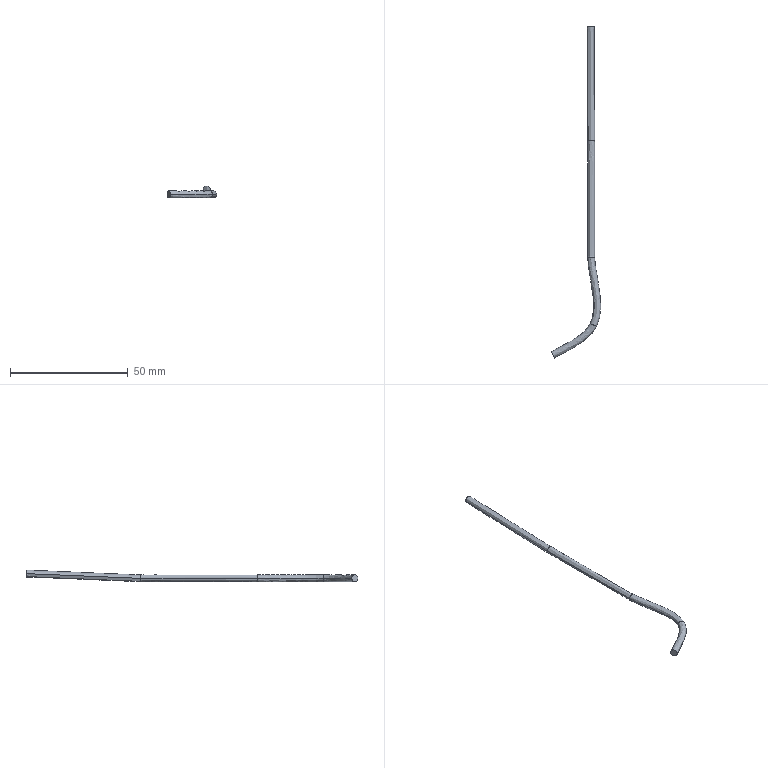Part | NX | features BREP 1 | 1 solid | 10 faces | box 21 x 141.003 x 5.012 mm | volume 1053 mm3 | spline 8 | plane 2